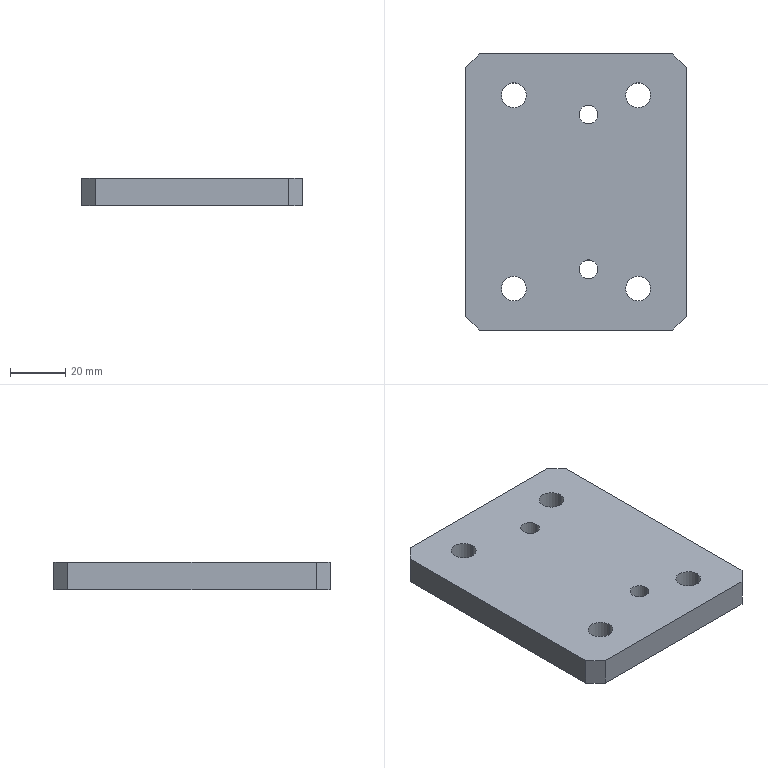Part | STEP file | 1 solid | 22 faces | box 80 x 100 x 10 mm | volume 76229 mm3 | cylinder 12 | plane 10 | commonest cylinder face diameters 9 x8 6.8 x4